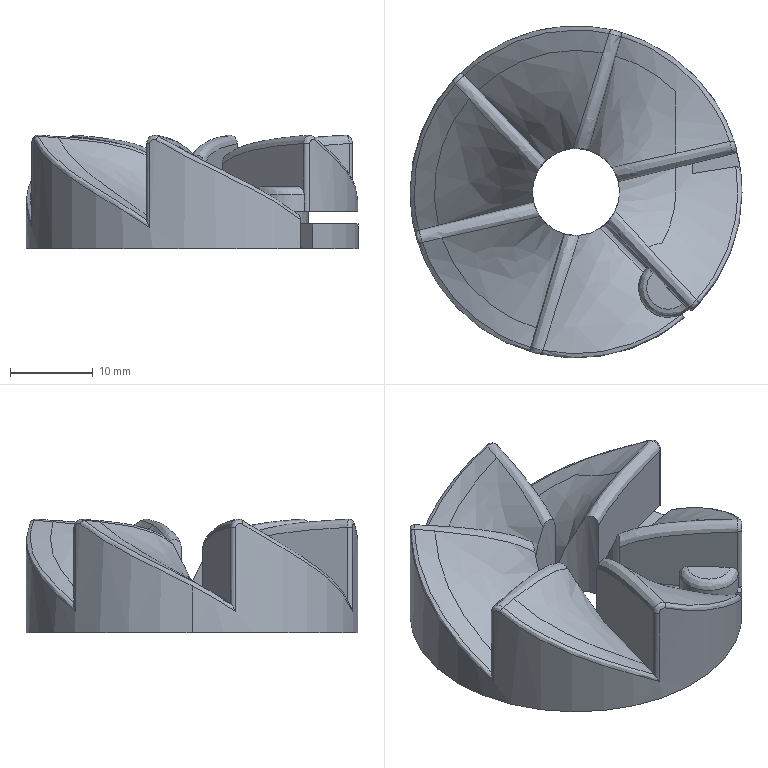Part | SolidWorks | features BaseBody 1 | 1 solid | 98 faces | box 40.118 x 40.118 x 13.737 mm | volume 8419 mm3 | spline 41 | cylinder 33 | plane 24 | commonest cylinder face diameters 1.003 x8 16.413 x6 34.235 x5 40.118 x5 4.062 x3 10.531 x2